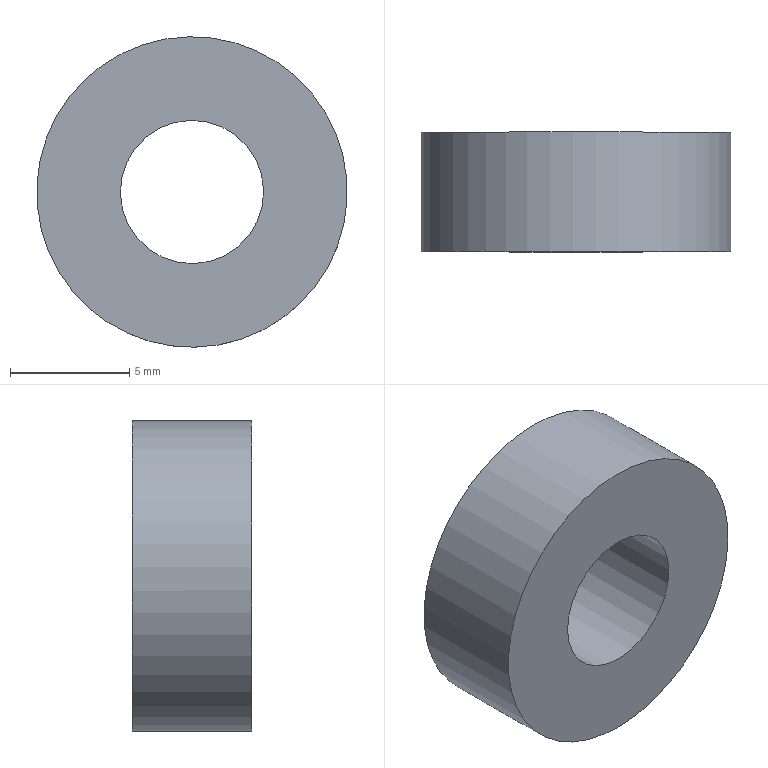Part | STEP file | Dodanie-wyci_gni_cie1_4 | 1 solid | 4 faces | box 13 x 5.005 x 13.002 mm | volume 522.29 mm3 | cylinder 2 | plane 2 | commonest cylinder face diameters 6 x1 13 x1
STEP:
#1=CARTESIAN_POINT('',(0.,0.,0.));
#2=DIRECTION('',(0.,0.,1.));
#3=DIRECTION('',(1.,0.,0.));
#4=AXIS2_PLACEMENT_3D('',#1,#2,#3);
#5=CARTESIAN_POINT('',(154.415,185.643,-126.524));
#6=VERTEX_POINT('',#5);
#7=CARTESIAN_POINT('',(154.415,180.643,-126.522));
#8=VERTEX_POINT('',#7);
#9=CARTESIAN_POINT('',(154.415,185.643,-126.524));
#10=DIRECTION('',(0.,-1.,0.0003815));
#11=VECTOR('',#10,1.);
#12=LINE('',#9,#11);
#13=CARTESIAN_POINT('',(160.724,180.644,-124.957));
#14=DIRECTION('',(0.,1.,-0.0003815));
#15=DIRECTION('',(-0.9706,-0.00009184,-0.2407));
#16=AXIS2_PLACEMENT_3D('',#13,#14,#15);
#17=CYLINDRICAL_SURFACE('',#16,6.5);
#18=CARTESIAN_POINT('',(0.,5.));
#19=DIRECTION('',(0.,-1.));
#20=VECTOR('',#19,1.);
#21=LINE('',#18,#20);
#22=(GEOMETRIC_REPRESENTATION_CONTEXT(2)PARAMETRIC_REPRESENTATION_CONTEXT()REPRESENTATION_CONTEXT('',''));
#23=DEFINITIONAL_REPRESENTATION('',(#21),#22);
#24=PCURVE('',#17,#23);
#25=CARTESIAN_POINT('',(6.283,5.));
#26=DIRECTION('',(0.,-1.));
#27=VECTOR('',#26,1.);
#28=LINE('',#25,#27);
#29=(GEOMETRIC_REPRESENTATION_CONTEXT(2)PARAMETRIC_REPRESENTATION_CONTEXT()REPRESENTATION_CONTEXT('',''));
#30=DEFINITIONAL_REPRESENTATION('',(#28),#29);
#31=PCURVE('',#17,#30);
#32=SEAM_CURVE('',#12,(#24,#31),.PCURVE_S1.);
#33=EDGE_CURVE('',#6,#8,#32,.T.);
#34=ORIENTED_EDGE('',*,*,#33,.T.);
#35=CARTESIAN_POINT('',(160.724,180.644,-124.957));
#36=DIRECTION('',(0.,1.,-0.0003815));
#37=DIRECTION('',(-0.9706,-0.00009184,-0.2407));
#38=AXIS2_PLACEMENT_3D('',#35,#36,#37);
#39=CIRCLE('',#38,6.5);
#40=CARTESIAN_POINT('',(0.,0.));
#41=DIRECTION('',(1.,0.));
#42=VECTOR('',#41,1.);
#43=LINE('',#40,#42);
#44=(GEOMETRIC_REPRESENTATION_CONTEXT(2)PARAMETRIC_REPRESENTATION_CONTEXT()REPRESENTATION_CONTEXT('',''));
#45=DEFINITIONAL_REPRESENTATION('',(#43),#44);
#46=PCURVE('',#17,#45);
#47=CARTESIAN_POINT('',(160.724,180.644,-124.957));
#48=DIRECTION('',(0.,-1.,0.0003815));
#49=DIRECTION('',(0.9706,0.00009184,0.2407));
#50=AXIS2_PLACEMENT_3D('',#47,#48,#49);
#51=PLANE('',#50);
#52=CARTESIAN_POINT('',(-6.5,0.));
#53=CARTESIAN_POINT('',(-6.5,11.258));
#54=CARTESIAN_POINT('',(3.25,5.629));
#55=CARTESIAN_POINT('',(13.,0.));
#56=CARTESIAN_POINT('',(3.25,-5.629));
#57=CARTESIAN_POINT('',(-6.5,-11.258));
#58=CARTESIAN_POINT('',(-6.5,0.));
#59=(BOUNDED_CURVE()B_SPLINE_CURVE(2,(#52,#53,#54,#55,#56,#57,#58),.UNSPECIFIED.,.T.,.F.)B_SPLINE_CURVE_WITH_KNOTS((1,2,2,2,2,1),(-2.094,0.,2.094,4.189,6.283,8.378),.UNSPECIFIED.)CURVE()GEOMETRIC_REPRESENTATION_ITEM()RATIONAL_B_SPLINE_CURVE((1.,0.5,1.,0.5,1.,0.5,1.))REPRESENTATION_ITEM(''));
#60=(GEOMETRIC_REPRESENTATION_CONTEXT(2)PARAMETRIC_REPRESENTATION_CONTEXT()REPRESENTATION_CONTEXT('',''));
#61=DEFINITIONAL_REPRESENTATION('',(#59),#60);
#62=PCURVE('',#51,#61);
#63=SURFACE_CURVE('',#39,(#46,#62),.PCURVE_S1.);
#64=EDGE_CURVE('',#8,#8,#63,.T.);
#65=ORIENTED_EDGE('',*,*,#64,.T.);
#66=ORIENTED_EDGE('',*,*,#33,.F.);
#67=CARTESIAN_POINT('',(160.724,185.644,-124.959));
#68=DIRECTION('',(0.,-1.,0.0003815));
#69=DIRECTION('',(-0.9706,-0.00009184,-0.2407));
#70=AXIS2_PLACEMENT_3D('',#67,#68,#69);
#71=CIRCLE('',#70,6.5);
#72=CARTESIAN_POINT('',(6.283,5.));
#73=DIRECTION('',(-1.,0.));
#74=VECTOR('',#73,1.);
#75=LINE('',#72,#74);
#76=(GEOMETRIC_REPRESENTATION_CONTEXT(2)PARAMETRIC_REPRESENTATION_CONTEXT()REPRESENTATION_CONTEXT('',''));
#77=DEFINITIONAL_REPRESENTATION('',(#75),#76);
#78=PCURVE('',#17,#77);
#79=CARTESIAN_POINT('',(160.724,185.644,-124.959));
#80=DIRECTION('',(0.,-1.,0.0003815));
#81=DIRECTION('',(0.9706,0.00009184,0.2407));
#82=AXIS2_PLACEMENT_3D('',#79,#80,#81);
#83=PLANE('',#82);
#84=CARTESIAN_POINT('',(0.,0.));
#85=DIRECTION('',(-1.,0.));
#86=AXIS2_PLACEMENT_2D('',#84,#85);
#87=CIRCLE('',#86,6.5);
#88=(GEOMETRIC_REPRESENTATION_CONTEXT(2)PARAMETRIC_REPRESENTATION_CONTEXT()REPRESENTATION_CONTEXT('',''));
#89=DEFINITIONAL_REPRESENTATION('',(#87),#88);
#90=PCURVE('',#83,#89);
#91=SURFACE_CURVE('',#71,(#78,#90),.PCURVE_S1.);
#92=EDGE_CURVE('',#6,#6,#91,.T.);
#93=ORIENTED_EDGE('',*,*,#92,.T.);
#94=EDGE_LOOP('',(#34,#65,#66,#93));
#95=FACE_BOUND('',#94,.T.);
#96=ADVANCED_FACE('',(#95),#17,.T.);
#97=CARTESIAN_POINT('',(157.812,180.644,-125.68));
#98=VERTEX_POINT('',#97);
#99=CARTESIAN_POINT('',(160.724,180.644,-124.957));
#100=DIRECTION('',(0.,1.,-0.0003815));
#101=DIRECTION('',(-0.9706,-0.00009184,-0.2407));
#102=AXIS2_PLACEMENT_3D('',#99,#100,#101);
#103=CIRCLE('',#102,3.);
#104=CARTESIAN_POINT('',(160.724,180.644,-124.957));
#105=DIRECTION('',(0.,1.,-0.0003815));
#106=DIRECTION('',(-0.9706,-0.00009184,-0.2407));
#107=AXIS2_PLACEMENT_3D('',#104,#105,#106);
#108=CYLINDRICAL_SURFACE('',#107,3.);
#109=CARTESIAN_POINT('',(0.,0.));
#110=DIRECTION('',(1.,0.));
#111=VECTOR('',#110,1.);
#112=LINE('',#109,#111);
#113=(GEOMETRIC_REPRESENTATION_CONTEXT(2)PARAMETRIC_REPRESENTATION_CONTEXT()REPRESENTATION_CONTEXT('',''));
#114=DEFINITIONAL_REPRESENTATION('',(#112),#113);
#115=PCURVE('',#108,#114);
#116=CARTESIAN_POINT('',(-3.,0.));
#117=CARTESIAN_POINT('',(-3.,5.196));
#118=CARTESIAN_POINT('',(1.5,2.598));
#119=CARTESIAN_POINT('',(6.,0.));
#120=CARTESIAN_POINT('',(1.5,-2.598));
#121=CARTESIAN_POINT('',(-3.,-5.196));
#122=CARTESIAN_POINT('',(-3.,0.));
#123=(BOUNDED_CURVE()B_SPLINE_CURVE(2,(#116,#117,#118,#119,#120,#121,#122),.UNSPECIFIED.,.T.,.F.)B_SPLINE_CURVE_WITH_KNOTS((1,2,2,2,2,1),(-2.094,0.,2.094,4.189,6.283,8.378),.UNSPECIFIED.)CURVE()GEOMETRIC_REPRESENTATION_ITEM()RATIONAL_B_SPLINE_CURVE((1.,0.5,1.,0.5,1.,0.5,1.))REPRESENTATION_ITEM(''));
#124=(GEOMETRIC_REPRESENTATION_CONTEXT(2)PARAMETRIC_REPRESENTATION_CONTEXT()REPRESENTATION_CONTEXT('',''));
#125=DEFINITIONAL_REPRESENTATION('',(#123),#124);
#126=PCURVE('',#51,#125);
#127=SURFACE_CURVE('',#103,(#115,#126),.PCURVE_S1.);
#128=EDGE_CURVE('',#98,#98,#127,.T.);
#129=ORIENTED_EDGE('',*,*,#128,.T.);
#130=CARTESIAN_POINT('',(157.812,185.644,-125.681));
#131=VERTEX_POINT('',#130);
#132=CARTESIAN_POINT('',(157.812,185.644,-125.681));
#133=DIRECTION('',(0.,-1.,0.0003815));
#134=VECTOR('',#133,1.);
#135=LINE('',#132,#134);
#136=CARTESIAN_POINT('',(6.283,5.));
#137=DIRECTION('',(0.,-1.));
#138=VECTOR('',#137,1.);
#139=LINE('',#136,#138);
#140=(GEOMETRIC_REPRESENTATION_CONTEXT(2)PARAMETRIC_REPRESENTATION_CONTEXT()REPRESENTATION_CONTEXT('',''));
#141=DEFINITIONAL_REPRESENTATION('',(#139),#140);
#142=PCURVE('',#108,#141);
#143=CARTESIAN_POINT('',(0.,5.));
#144=DIRECTION('',(0.,-1.));
#145=VECTOR('',#144,1.);
#146=LINE('',#143,#145);
#147=(GEOMETRIC_REPRESENTATION_CONTEXT(2)PARAMETRIC_REPRESENTATION_CONTEXT()REPRESENTATION_CONTEXT('',''));
#148=DEFINITIONAL_REPRESENTATION('',(#146),#147);
#149=PCURVE('',#108,#148);
#150=SEAM_CURVE('',#135,(#142,#149),.PCURVE_S1.);
#151=EDGE_CURVE('',#131,#98,#150,.T.);
#152=ORIENTED_EDGE('',*,*,#151,.F.);
#153=CARTESIAN_POINT('',(160.724,185.644,-124.959));
#154=DIRECTION('',(0.,1.,-0.0003815));
#155=DIRECTION('',(-0.9706,-0.00009184,-0.2407));
#156=AXIS2_PLACEMENT_3D('',#153,#154,#155);
#157=CIRCLE('',#156,3.);
#158=CARTESIAN_POINT('',(0.,5.));
#159=DIRECTION('',(1.,0.));
#160=VECTOR('',#159,1.);
#161=LINE('',#158,#160);
#162=(GEOMETRIC_REPRESENTATION_CONTEXT(2)PARAMETRIC_REPRESENTATION_CONTEXT()REPRESENTATION_CONTEXT('',''));
#163=DEFINITIONAL_REPRESENTATION('',(#161),#162);
#164=PCURVE('',#108,#163);
#165=CARTESIAN_POINT('',(-3.,0.));
#166=CARTESIAN_POINT('',(-3.,5.196));
#167=CARTESIAN_POINT('',(1.5,2.598));
#168=CARTESIAN_POINT('',(6.,0.));
#169=CARTESIAN_POINT('',(1.5,-2.598));
#170=CARTESIAN_POINT('',(-3.,-5.196));
#171=CARTESIAN_POINT('',(-3.,0.));
#172=(BOUNDED_CURVE()B_SPLINE_CURVE(2,(#165,#166,#167,#168,#169,#170,#171),.UNSPECIFIED.,.T.,.F.)B_SPLINE_CURVE_WITH_KNOTS((1,2,2,2,2,1),(-2.094,0.,2.094,4.189,6.283,8.378),.UNSPECIFIED.)CURVE()GEOMETRIC_REPRESENTATION_ITEM()RATIONAL_B_SPLINE_CURVE((1.,0.5,1.,0.5,1.,0.5,1.))REPRESENTATION_ITEM(''));
#173=(GEOMETRIC_REPRESENTATION_CONTEXT(2)PARAMETRIC_REPRESENTATION_CONTEXT()REPRESENTATION_CONTEXT('',''));
#174=DEFINITIONAL_REPRESENTATION('',(#172),#173);
#175=PCURVE('',#83,#174);
#176=SURFACE_CURVE('',#157,(#164,#175),.PCURVE_S1.);
#177=EDGE_CURVE('',#131,#131,#176,.T.);
#178=ORIENTED_EDGE('',*,*,#177,.F.);
#179=ORIENTED_EDGE('',*,*,#151,.T.);
#180=EDGE_LOOP('',(#129,#152,#178,#179));
#181=FACE_BOUND('',#180,.F.);
#182=ADVANCED_FACE('',(#181),#108,.F.);
#183=ORIENTED_EDGE('',*,*,#177,.F.);
#184=EDGE_LOOP('',(#183));
#185=FACE_BOUND('',#184,.T.);
#186=ORIENTED_EDGE('',*,*,#92,.F.);
#187=EDGE_LOOP('',(#186));
#188=FACE_BOUND('',#187,.T.);
#189=ADVANCED_FACE('',(#185,#188),#83,.F.);
#190=ORIENTED_EDGE('',*,*,#128,.T.);
#191=EDGE_LOOP('',(#190));
#192=FACE_BOUND('',#191,.T.);
#193=ORIENTED_EDGE('',*,*,#64,.F.);
#194=EDGE_LOOP('',(#193));
#195=FACE_BOUND('',#194,.T.);
#196=ADVANCED_FACE('',(#192,#195),#51,.T.);
#197=CLOSED_SHELL('',(#96,#182,#189,#196));
#198=MANIFOLD_SOLID_BREP('',#197);
#199=(LENGTH_UNIT()NAMED_UNIT(*)SI_UNIT(.MILLI.,.METRE.));
#200=UNCERTAINTY_MEASURE_WITH_UNIT(LENGTH_MEASURE(0.0000001),#199,'','');
#201=(NAMED_UNIT(*)PLANE_ANGLE_UNIT()SI_UNIT($,.RADIAN.));
#202=(NAMED_UNIT(*)SI_UNIT($,.STERADIAN.)SOLID_ANGLE_UNIT());
#203=(GEOMETRIC_REPRESENTATION_CONTEXT(3)GLOBAL_UNCERTAINTY_ASSIGNED_CONTEXT((#200))GLOBAL_UNIT_ASSIGNED_CONTEXT((#199,#201,#202))REPRESENTATION_CONTEXT('',''));
#204=ADVANCED_BREP_SHAPE_REPRESENTATION('',(#4,#198),#203);